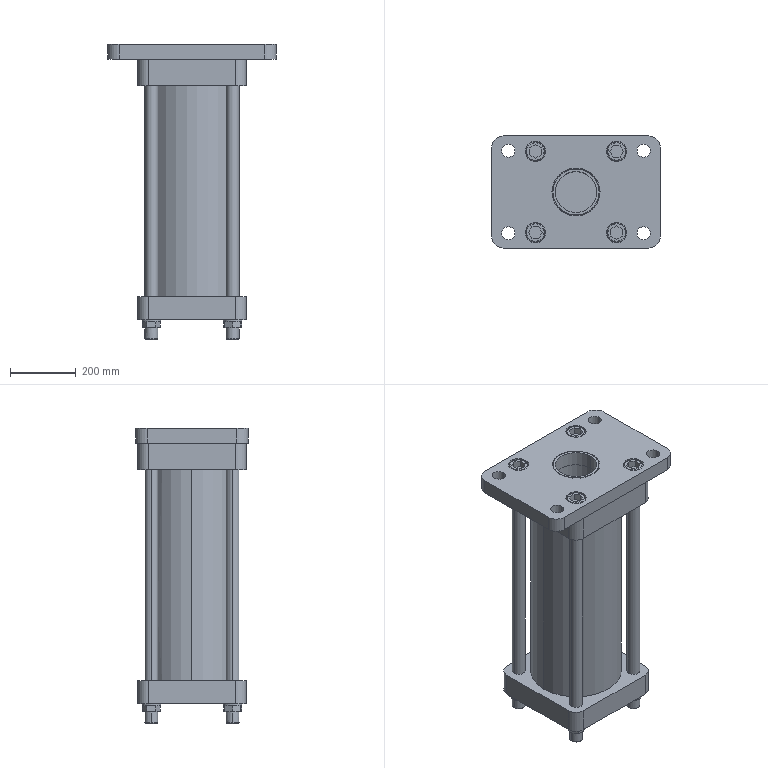Part | SolidWorks | features BaseBody 7 | 7 solids | 622 faces | box 510 x 340 x 894.436 mm | volume 57179698 mm3 | plane 258 | spline 204 | cylinder 126 | cone 34 | commonest cylinder face diameters 39 x32 275.02 x26 275 x12 40 x8 56.16 x8 58.5 x8